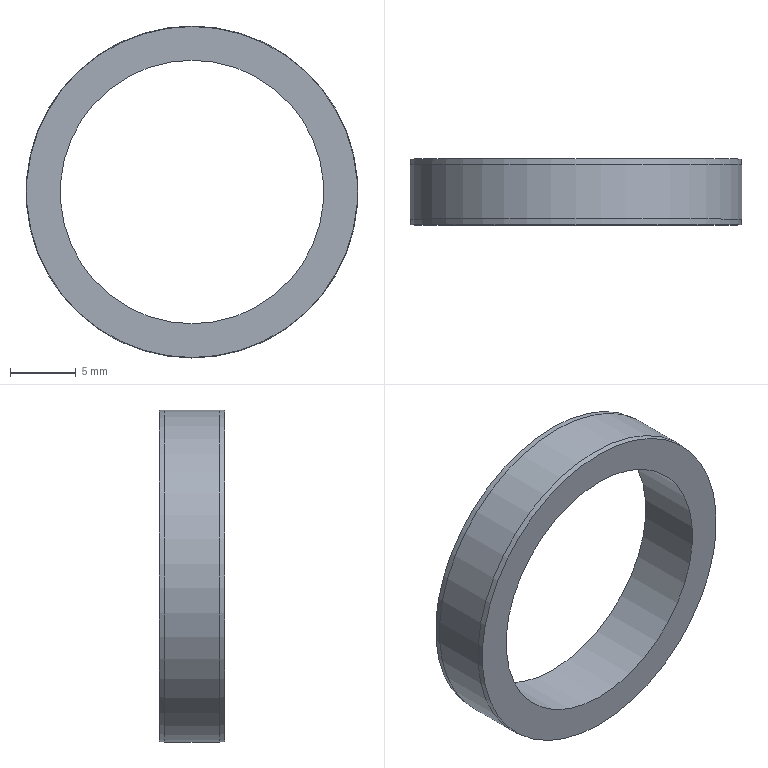Part | STEP file | 2-06.2 | 1 solid | 6 faces | box 25.2 x 5 x 25.2 mm | volume 921.7 mm3 | cylinder 2 | plane 2 | cone 2 | commonest cylinder face diameters 20 x1 25.2 x1
STEP:
#1=CARTESIAN_POINT('',(0.,0.,0.));
#2=DIRECTION('',(0.,0.,1.));
#3=DIRECTION('',(1.,0.,0.));
#4=AXIS2_PLACEMENT_3D('',#1,#2,#3);
#5=CARTESIAN_POINT('',(0.,0.,10.));
#6=VERTEX_POINT('',#5);
#7=CARTESIAN_POINT('',(0.,0.,0.));
#8=DIRECTION('',(0.,1.,0.));
#9=DIRECTION('',(0.,0.,1.));
#10=AXIS2_PLACEMENT_3D('',#7,#8,#9);
#11=CIRCLE('',#10,10.);
#12=CARTESIAN_POINT('',(0.,0.,0.));
#13=DIRECTION('',(0.,1.,0.));
#14=DIRECTION('',(0.,0.,1.));
#15=AXIS2_PLACEMENT_3D('',#12,#13,#14);
#16=CYLINDRICAL_SURFACE('',#15,10.);
#17=CARTESIAN_POINT('',(0.,0.));
#18=DIRECTION('',(1.,0.));
#19=VECTOR('',#18,1.);
#20=LINE('',#17,#19);
#21=(GEOMETRIC_REPRESENTATION_CONTEXT(2)PARAMETRIC_REPRESENTATION_CONTEXT()REPRESENTATION_CONTEXT('',''));
#22=DEFINITIONAL_REPRESENTATION('',(#20),#21);
#23=PCURVE('',#16,#22);
#24=CARTESIAN_POINT('',(0.,0.,0.));
#25=DIRECTION('',(0.,-1.,0.));
#26=DIRECTION('',(0.,0.,1.));
#27=AXIS2_PLACEMENT_3D('',#24,#25,#26);
#28=PLANE('',#27);
#29=CARTESIAN_POINT('',(10.,0.));
#30=CARTESIAN_POINT('',(10.,-17.321));
#31=CARTESIAN_POINT('',(-5.,-8.66));
#32=CARTESIAN_POINT('',(-20.,0.));
#33=CARTESIAN_POINT('',(-5.,8.66));
#34=CARTESIAN_POINT('',(10.,17.321));
#35=CARTESIAN_POINT('',(10.,0.));
#36=(BOUNDED_CURVE()B_SPLINE_CURVE(2,(#29,#30,#31,#32,#33,#34,#35),.UNSPECIFIED.,.T.,.F.)B_SPLINE_CURVE_WITH_KNOTS((1,2,2,2,2,1),(-2.094,0.,2.094,4.189,6.283,8.378),.UNSPECIFIED.)CURVE()GEOMETRIC_REPRESENTATION_ITEM()RATIONAL_B_SPLINE_CURVE((1.,0.5,1.,0.5,1.,0.5,1.))REPRESENTATION_ITEM(''));
#37=(GEOMETRIC_REPRESENTATION_CONTEXT(2)PARAMETRIC_REPRESENTATION_CONTEXT()REPRESENTATION_CONTEXT('',''));
#38=DEFINITIONAL_REPRESENTATION('',(#36),#37);
#39=PCURVE('',#28,#38);
#40=SURFACE_CURVE('',#11,(#23,#39),.PCURVE_S1.);
#41=EDGE_CURVE('',#6,#6,#40,.T.);
#42=ORIENTED_EDGE('',*,*,#41,.T.);
#43=CARTESIAN_POINT('',(0.,5.,10.));
#44=VERTEX_POINT('',#43);
#45=CARTESIAN_POINT('',(0.,0.,10.));
#46=DIRECTION('',(0.,1.,0.));
#47=VECTOR('',#46,1.);
#48=LINE('',#45,#47);
#49=CARTESIAN_POINT('',(6.283,0.));
#50=DIRECTION('',(0.,1.));
#51=VECTOR('',#50,1.);
#52=LINE('',#49,#51);
#53=(GEOMETRIC_REPRESENTATION_CONTEXT(2)PARAMETRIC_REPRESENTATION_CONTEXT()REPRESENTATION_CONTEXT('',''));
#54=DEFINITIONAL_REPRESENTATION('',(#52),#53);
#55=PCURVE('',#16,#54);
#56=CARTESIAN_POINT('',(0.,0.));
#57=DIRECTION('',(0.,1.));
#58=VECTOR('',#57,1.);
#59=LINE('',#56,#58);
#60=(GEOMETRIC_REPRESENTATION_CONTEXT(2)PARAMETRIC_REPRESENTATION_CONTEXT()REPRESENTATION_CONTEXT('',''));
#61=DEFINITIONAL_REPRESENTATION('',(#59),#60);
#62=PCURVE('',#16,#61);
#63=SEAM_CURVE('',#48,(#55,#62),.PCURVE_S1.);
#64=EDGE_CURVE('',#6,#44,#63,.T.);
#65=ORIENTED_EDGE('',*,*,#64,.T.);
#66=CARTESIAN_POINT('',(0.,5.,0.));
#67=DIRECTION('',(0.,1.,0.));
#68=DIRECTION('',(0.,0.,1.));
#69=AXIS2_PLACEMENT_3D('',#66,#67,#68);
#70=CIRCLE('',#69,10.);
#71=CARTESIAN_POINT('',(0.,5.));
#72=DIRECTION('',(1.,0.));
#73=VECTOR('',#72,1.);
#74=LINE('',#71,#73);
#75=(GEOMETRIC_REPRESENTATION_CONTEXT(2)PARAMETRIC_REPRESENTATION_CONTEXT()REPRESENTATION_CONTEXT('',''));
#76=DEFINITIONAL_REPRESENTATION('',(#74),#75);
#77=PCURVE('',#16,#76);
#78=CARTESIAN_POINT('',(0.,5.,0.));
#79=DIRECTION('',(0.,1.,0.));
#80=DIRECTION('',(0.,0.,1.));
#81=AXIS2_PLACEMENT_3D('',#78,#79,#80);
#82=PLANE('',#81);
#83=CARTESIAN_POINT('',(0.,0.));
#84=DIRECTION('',(1.,0.));
#85=AXIS2_PLACEMENT_2D('',#83,#84);
#86=CIRCLE('',#85,10.);
#87=(GEOMETRIC_REPRESENTATION_CONTEXT(2)PARAMETRIC_REPRESENTATION_CONTEXT()REPRESENTATION_CONTEXT('',''));
#88=DEFINITIONAL_REPRESENTATION('',(#86),#87);
#89=PCURVE('',#82,#88);
#90=SURFACE_CURVE('',#70,(#77,#89),.PCURVE_S1.);
#91=EDGE_CURVE('',#44,#44,#90,.T.);
#92=ORIENTED_EDGE('',*,*,#91,.F.);
#93=ORIENTED_EDGE('',*,*,#64,.F.);
#94=EDGE_LOOP('',(#42,#65,#92,#93));
#95=FACE_BOUND('',#94,.F.);
#96=ADVANCED_FACE('',(#95),#16,.F.);
#97=CARTESIAN_POINT('',(0.,5.,12.563));
#98=VERTEX_POINT('',#97);
#99=CARTESIAN_POINT('',(0.,5.,0.));
#100=DIRECTION('',(0.,1.,0.));
#101=DIRECTION('',(0.,0.,1.));
#102=AXIS2_PLACEMENT_3D('',#99,#100,#101);
#103=CIRCLE('',#102,12.563);
#104=CARTESIAN_POINT('',(0.,0.));
#105=DIRECTION('',(1.,0.));
#106=AXIS2_PLACEMENT_2D('',#104,#105);
#107=CIRCLE('',#106,12.563);
#108=(GEOMETRIC_REPRESENTATION_CONTEXT(2)PARAMETRIC_REPRESENTATION_CONTEXT()REPRESENTATION_CONTEXT('',''));
#109=DEFINITIONAL_REPRESENTATION('',(#107),#108);
#110=PCURVE('',#82,#109);
#111=CARTESIAN_POINT('',(0.,5.,0.));
#112=DIRECTION('',(0.,-1.,0.));
#113=DIRECTION('',(0.,0.,1.));
#114=AXIS2_PLACEMENT_3D('',#111,#112,#113);
#115=CONICAL_SURFACE('',#114,12.563,0.08472);
#116=CARTESIAN_POINT('',(6.283,0.));
#117=DIRECTION('',(-1.,0.));
#118=VECTOR('',#117,1.);
#119=LINE('',#116,#118);
#120=(GEOMETRIC_REPRESENTATION_CONTEXT(2)PARAMETRIC_REPRESENTATION_CONTEXT()REPRESENTATION_CONTEXT('',''));
#121=DEFINITIONAL_REPRESENTATION('',(#119),#120);
#122=PCURVE('',#115,#121);
#123=SURFACE_CURVE('',#103,(#110,#122),.PCURVE_S1.);
#124=EDGE_CURVE('',#98,#98,#123,.T.);
#125=ORIENTED_EDGE('',*,*,#124,.T.);
#126=EDGE_LOOP('',(#125));
#127=FACE_BOUND('',#126,.T.);
#128=ORIENTED_EDGE('',*,*,#91,.F.);
#129=EDGE_LOOP('',(#128));
#130=FACE_BOUND('',#129,.T.);
#131=ADVANCED_FACE('',(#127,#130),#82,.T.);
#132=CARTESIAN_POINT('',(0.,4.56,12.6));
#133=VERTEX_POINT('',#132);
#134=CARTESIAN_POINT('',(0.,5.,12.563));
#135=DIRECTION('',(0.,-0.9964,0.08462));
#136=VECTOR('',#135,1.);
#137=LINE('',#134,#136);
#138=CARTESIAN_POINT('',(6.283,0.));
#139=DIRECTION('',(0.,1.));
#140=VECTOR('',#139,1.);
#141=LINE('',#138,#140);
#142=(GEOMETRIC_REPRESENTATION_CONTEXT(2)PARAMETRIC_REPRESENTATION_CONTEXT()REPRESENTATION_CONTEXT('',''));
#143=DEFINITIONAL_REPRESENTATION('',(#141),#142);
#144=PCURVE('',#115,#143);
#145=CARTESIAN_POINT('',(0.,0.));
#146=DIRECTION('',(0.,1.));
#147=VECTOR('',#146,1.);
#148=LINE('',#145,#147);
#149=(GEOMETRIC_REPRESENTATION_CONTEXT(2)PARAMETRIC_REPRESENTATION_CONTEXT()REPRESENTATION_CONTEXT('',''));
#150=DEFINITIONAL_REPRESENTATION('',(#148),#149);
#151=PCURVE('',#115,#150);
#152=SEAM_CURVE('',#137,(#144,#151),.PCURVE_S1.);
#153=EDGE_CURVE('',#98,#133,#152,.T.);
#154=ORIENTED_EDGE('',*,*,#153,.T.);
#155=CARTESIAN_POINT('',(0.,4.56,0.));
#156=DIRECTION('',(0.,1.,0.));
#157=DIRECTION('',(0.,0.,1.));
#158=AXIS2_PLACEMENT_3D('',#155,#156,#157);
#159=CIRCLE('',#158,12.6);
#160=CARTESIAN_POINT('',(6.283,0.4399));
#161=DIRECTION('',(-1.,0.));
#162=VECTOR('',#161,1.);
#163=LINE('',#160,#162);
#164=(GEOMETRIC_REPRESENTATION_CONTEXT(2)PARAMETRIC_REPRESENTATION_CONTEXT()REPRESENTATION_CONTEXT('',''));
#165=DEFINITIONAL_REPRESENTATION('',(#163),#164);
#166=PCURVE('',#115,#165);
#167=CARTESIAN_POINT('',(0.,4.56,0.));
#168=DIRECTION('',(0.,-1.,0.));
#169=DIRECTION('',(0.,0.,1.));
#170=AXIS2_PLACEMENT_3D('',#167,#168,#169);
#171=CYLINDRICAL_SURFACE('',#170,12.6);
#172=CARTESIAN_POINT('',(6.283,0.));
#173=DIRECTION('',(-1.,0.));
#174=VECTOR('',#173,1.);
#175=LINE('',#172,#174);
#176=(GEOMETRIC_REPRESENTATION_CONTEXT(2)PARAMETRIC_REPRESENTATION_CONTEXT()REPRESENTATION_CONTEXT('',''));
#177=DEFINITIONAL_REPRESENTATION('',(#175),#176);
#178=PCURVE('',#171,#177);
#179=SURFACE_CURVE('',#159,(#166,#178),.PCURVE_S1.);
#180=EDGE_CURVE('',#133,#133,#179,.T.);
#181=ORIENTED_EDGE('',*,*,#180,.T.);
#182=ORIENTED_EDGE('',*,*,#153,.F.);
#183=ORIENTED_EDGE('',*,*,#124,.F.);
#184=EDGE_LOOP('',(#154,#181,#182,#183));
#185=FACE_BOUND('',#184,.T.);
#186=ADVANCED_FACE('',(#185),#115,.T.);
#187=CARTESIAN_POINT('',(0.,0.4399,12.6));
#188=VERTEX_POINT('',#187);
#189=CARTESIAN_POINT('',(0.,4.56,12.6));
#190=DIRECTION('',(0.,-1.,0.));
#191=VECTOR('',#190,1.);
#192=LINE('',#189,#191);
#193=CARTESIAN_POINT('',(6.283,0.));
#194=DIRECTION('',(0.,1.));
#195=VECTOR('',#194,1.);
#196=LINE('',#193,#195);
#197=(GEOMETRIC_REPRESENTATION_CONTEXT(2)PARAMETRIC_REPRESENTATION_CONTEXT()REPRESENTATION_CONTEXT('',''));
#198=DEFINITIONAL_REPRESENTATION('',(#196),#197);
#199=PCURVE('',#171,#198);
#200=CARTESIAN_POINT('',(0.,0.));
#201=DIRECTION('',(0.,1.));
#202=VECTOR('',#201,1.);
#203=LINE('',#200,#202);
#204=(GEOMETRIC_REPRESENTATION_CONTEXT(2)PARAMETRIC_REPRESENTATION_CONTEXT()REPRESENTATION_CONTEXT('',''));
#205=DEFINITIONAL_REPRESENTATION('',(#203),#204);
#206=PCURVE('',#171,#205);
#207=SEAM_CURVE('',#192,(#199,#206),.PCURVE_S1.);
#208=EDGE_CURVE('',#133,#188,#207,.T.);
#209=ORIENTED_EDGE('',*,*,#208,.T.);
#210=CARTESIAN_POINT('',(0.,0.4399,0.));
#211=DIRECTION('',(0.,1.,0.));
#212=DIRECTION('',(0.,0.,1.));
#213=AXIS2_PLACEMENT_3D('',#210,#211,#212);
#214=CIRCLE('',#213,12.6);
#215=CARTESIAN_POINT('',(6.283,4.12));
#216=DIRECTION('',(-1.,0.));
#217=VECTOR('',#216,1.);
#218=LINE('',#215,#217);
#219=(GEOMETRIC_REPRESENTATION_CONTEXT(2)PARAMETRIC_REPRESENTATION_CONTEXT()REPRESENTATION_CONTEXT('',''));
#220=DEFINITIONAL_REPRESENTATION('',(#218),#219);
#221=PCURVE('',#171,#220);
#222=CARTESIAN_POINT('',(0.,0.,0.));
#223=DIRECTION('',(0.,1.,0.));
#224=DIRECTION('',(0.,0.,1.));
#225=AXIS2_PLACEMENT_3D('',#222,#223,#224);
#226=CONICAL_SURFACE('',#225,12.563,0.08472);
#227=CARTESIAN_POINT('',(0.,0.4399));
#228=DIRECTION('',(1.,0.));
#229=VECTOR('',#228,1.);
#230=LINE('',#227,#229);
#231=(GEOMETRIC_REPRESENTATION_CONTEXT(2)PARAMETRIC_REPRESENTATION_CONTEXT()REPRESENTATION_CONTEXT('',''));
#232=DEFINITIONAL_REPRESENTATION('',(#230),#231);
#233=PCURVE('',#226,#232);
#234=SURFACE_CURVE('',#214,(#221,#233),.PCURVE_S1.);
#235=EDGE_CURVE('',#188,#188,#234,.T.);
#236=ORIENTED_EDGE('',*,*,#235,.T.);
#237=ORIENTED_EDGE('',*,*,#208,.F.);
#238=ORIENTED_EDGE('',*,*,#180,.F.);
#239=EDGE_LOOP('',(#209,#236,#237,#238));
#240=FACE_BOUND('',#239,.T.);
#241=ADVANCED_FACE('',(#240),#171,.T.);
#242=CARTESIAN_POINT('',(0.,0.,12.563));
#243=VERTEX_POINT('',#242);
#244=CARTESIAN_POINT('',(0.,0.4399,12.6));
#245=DIRECTION('',(0.,-0.9964,-0.08462));
#246=VECTOR('',#245,1.);
#247=LINE('',#244,#246);
#248=CARTESIAN_POINT('',(0.,0.4399));
#249=DIRECTION('',(0.,-1.));
#250=VECTOR('',#249,1.);
#251=LINE('',#248,#250);
#252=(GEOMETRIC_REPRESENTATION_CONTEXT(2)PARAMETRIC_REPRESENTATION_CONTEXT()REPRESENTATION_CONTEXT('',''));
#253=DEFINITIONAL_REPRESENTATION('',(#251),#252);
#254=PCURVE('',#226,#253);
#255=CARTESIAN_POINT('',(6.283,0.4399));
#256=DIRECTION('',(0.,-1.));
#257=VECTOR('',#256,1.);
#258=LINE('',#255,#257);
#259=(GEOMETRIC_REPRESENTATION_CONTEXT(2)PARAMETRIC_REPRESENTATION_CONTEXT()REPRESENTATION_CONTEXT('',''));
#260=DEFINITIONAL_REPRESENTATION('',(#258),#259);
#261=PCURVE('',#226,#260);
#262=SEAM_CURVE('',#247,(#254,#261),.PCURVE_S1.);
#263=EDGE_CURVE('',#188,#243,#262,.T.);
#264=ORIENTED_EDGE('',*,*,#263,.T.);
#265=CARTESIAN_POINT('',(0.,0.,0.));
#266=DIRECTION('',(0.,1.,0.));
#267=DIRECTION('',(0.,0.,1.));
#268=AXIS2_PLACEMENT_3D('',#265,#266,#267);
#269=CIRCLE('',#268,12.563);
#270=CARTESIAN_POINT('',(0.,0.));
#271=DIRECTION('',(1.,0.));
#272=VECTOR('',#271,1.);
#273=LINE('',#270,#272);
#274=(GEOMETRIC_REPRESENTATION_CONTEXT(2)PARAMETRIC_REPRESENTATION_CONTEXT()REPRESENTATION_CONTEXT('',''));
#275=DEFINITIONAL_REPRESENTATION('',(#273),#274);
#276=PCURVE('',#226,#275);
#277=CARTESIAN_POINT('',(12.563,0.));
#278=CARTESIAN_POINT('',(12.563,-21.759));
#279=CARTESIAN_POINT('',(-6.281,-10.88));
#280=CARTESIAN_POINT('',(-25.125,0.));
#281=CARTESIAN_POINT('',(-6.281,10.88));
#282=CARTESIAN_POINT('',(12.563,21.759));
#283=CARTESIAN_POINT('',(12.563,0.));
#284=(BOUNDED_CURVE()B_SPLINE_CURVE(2,(#277,#278,#279,#280,#281,#282,#283),.UNSPECIFIED.,.T.,.F.)B_SPLINE_CURVE_WITH_KNOTS((1,2,2,2,2,1),(-2.094,0.,2.094,4.189,6.283,8.378),.UNSPECIFIED.)CURVE()GEOMETRIC_REPRESENTATION_ITEM()RATIONAL_B_SPLINE_CURVE((1.,0.5,1.,0.5,1.,0.5,1.))REPRESENTATION_ITEM(''));
#285=(GEOMETRIC_REPRESENTATION_CONTEXT(2)PARAMETRIC_REPRESENTATION_CONTEXT()REPRESENTATION_CONTEXT('',''));
#286=DEFINITIONAL_REPRESENTATION('',(#284),#285);
#287=PCURVE('',#28,#286);
#288=SURFACE_CURVE('',#269,(#276,#287),.PCURVE_S1.);
#289=EDGE_CURVE('',#243,#243,#288,.T.);
#290=ORIENTED_EDGE('',*,*,#289,.T.);
#291=ORIENTED_EDGE('',*,*,#263,.F.);
#292=ORIENTED_EDGE('',*,*,#235,.F.);
#293=EDGE_LOOP('',(#264,#290,#291,#292));
#294=FACE_BOUND('',#293,.T.);
#295=ADVANCED_FACE('',(#294),#226,.T.);
#296=ORIENTED_EDGE('',*,*,#289,.F.);
#297=EDGE_LOOP('',(#296));
#298=FACE_BOUND('',#297,.T.);
#299=ORIENTED_EDGE('',*,*,#41,.T.);
#300=EDGE_LOOP('',(#299));
#301=FACE_BOUND('',#300,.T.);
#302=ADVANCED_FACE('',(#298,#301),#28,.T.);
#303=CLOSED_SHELL('',(#96,#131,#186,#241,#295,#302));
#304=MANIFOLD_SOLID_BREP('',#303);
#305=(LENGTH_UNIT()NAMED_UNIT(*)SI_UNIT(.MILLI.,.METRE.));
#306=UNCERTAINTY_MEASURE_WITH_UNIT(LENGTH_MEASURE(0.0000001),#305,'','');
#307=(NAMED_UNIT(*)PLANE_ANGLE_UNIT()SI_UNIT($,.RADIAN.));
#308=(NAMED_UNIT(*)SI_UNIT($,.STERADIAN.)SOLID_ANGLE_UNIT());
#309=(GEOMETRIC_REPRESENTATION_CONTEXT(3)GLOBAL_UNCERTAINTY_ASSIGNED_CONTEXT((#306))GLOBAL_UNIT_ASSIGNED_CONTEXT((#305,#307,#308))REPRESENTATION_CONTEXT('',''));
#310=ADVANCED_BREP_SHAPE_REPRESENTATION('',(#4,#304),#309);